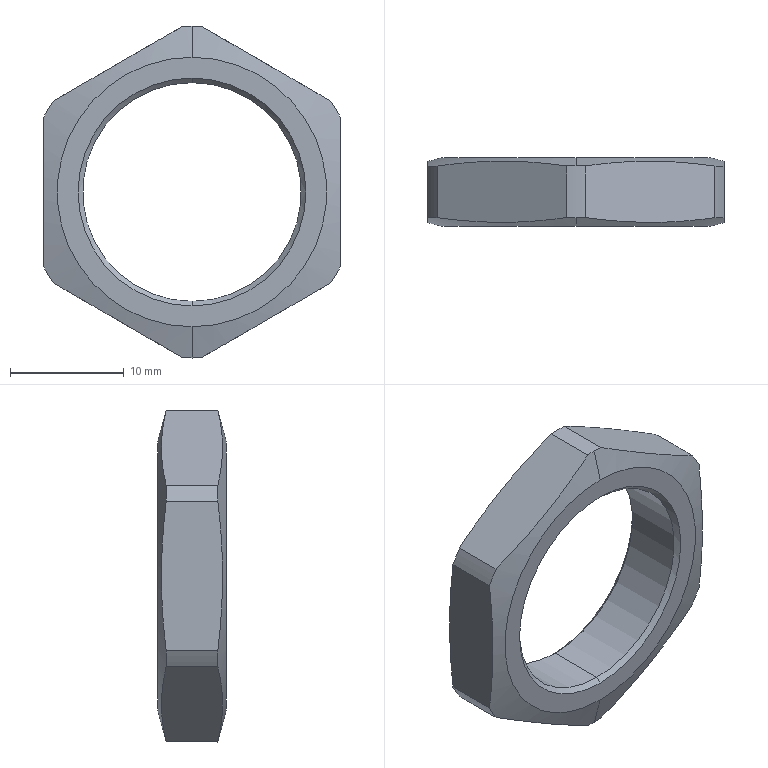Part | SolidWorks | features BaseBody 1 | 1 solid | 25 faces | box 26 x 6 x 29.132 mm | volume 1676 mm3 | cylinder 9 | cone 8 | plane 8 | commonest cylinder face diameters 29.132 x7 19.188 x2
STEP:
#1=CARTESIAN_POINT('',(0.,6.,-11.818));
#2=VERTEX_POINT('',#1);
#3=CARTESIAN_POINT('',(0.,6.,11.818));
#4=VERTEX_POINT('',#3);
#5=CARTESIAN_POINT('',(0.,6.,0.));
#6=DIRECTION('',(0.,-1.,0.));
#7=DIRECTION('',(0.,0.,-1.));
#8=AXIS2_PLACEMENT_3D('',#5,#6,#7);
#9=CIRCLE('',#8,11.818);
#10=EDGE_CURVE('',#2,#4,#9,.T.);
#11=ORIENTED_EDGE('',*,*,#10,.T.);
#12=CARTESIAN_POINT('',(0.,5.264,14.566));
#13=VERTEX_POINT('',#12);
#14=CARTESIAN_POINT('',(0.,3.,23.014));
#15=DIRECTION('',(0.,-0.2588,0.9659));
#16=VECTOR('',#15,1000.);
#17=LINE('',#14,#16);
#18=EDGE_CURVE('',#4,#13,#17,.T.);
#19=ORIENTED_EDGE('',*,*,#18,.T.);
#20=CARTESIAN_POINT('',(0.8103,5.264,14.543));
#21=VERTEX_POINT('',#20);
#22=CARTESIAN_POINT('',(0.,5.264,0.));
#23=DIRECTION('',(0.,-1.,0.));
#24=DIRECTION('',(0.,0.,-1.));
#25=AXIS2_PLACEMENT_3D('',#22,#23,#24);
#26=CIRCLE('',#25,14.566);
#27=EDGE_CURVE('',#21,#13,#26,.T.);
#28=ORIENTED_EDGE('',*,*,#27,.F.);
#29=CARTESIAN_POINT('',(12.19,5.264,7.973));
#30=VERTEX_POINT('',#29);
#31=CARTESIAN_POINT('',(12.19,5.264,7.973));
#32=CARTESIAN_POINT('',(11.241,5.396,8.521));
#33=CARTESIAN_POINT('',(10.293,5.502,9.068));
#34=CARTESIAN_POINT('',(8.397,5.646,10.163));
#35=CARTESIAN_POINT('',(6.5,5.721,11.258));
#36=CARTESIAN_POINT('',(4.603,5.646,12.353));
#37=CARTESIAN_POINT('',(2.707,5.502,13.448));
#38=CARTESIAN_POINT('',(1.759,5.396,13.996));
#39=CARTESIAN_POINT('',(0.8103,5.264,14.543));
#40=B_SPLINE_CURVE_WITH_KNOTS('',3,(#31,#32,#33,#34,#35,#36,#37,#38,#39),.UNSPECIFIED.,.F.,.F.,(4,2,1,2,4),(0.,0.003285,0.00657,0.009855,0.01314),.UNSPECIFIED.);
#41=EDGE_CURVE('',#30,#21,#40,.T.);
#42=ORIENTED_EDGE('',*,*,#41,.F.);
#43=CARTESIAN_POINT('',(13.,5.264,6.57));
#44=VERTEX_POINT('',#43);
#45=CARTESIAN_POINT('',(0.,5.264,0.));
#46=DIRECTION('',(0.,-1.,0.));
#47=DIRECTION('',(0.,0.,-1.));
#48=AXIS2_PLACEMENT_3D('',#45,#46,#47);
#49=CIRCLE('',#48,14.566);
#50=EDGE_CURVE('',#44,#30,#49,.T.);
#51=ORIENTED_EDGE('',*,*,#50,.F.);
#52=CARTESIAN_POINT('',(13.,5.264,-6.57));
#53=VERTEX_POINT('',#52);
#54=CARTESIAN_POINT('',(13.,5.264,-6.57));
#55=CARTESIAN_POINT('',(13.,5.396,-5.475));
#56=CARTESIAN_POINT('',(13.,5.502,-4.38));
#57=CARTESIAN_POINT('',(13.,5.646,-2.19));
#58=CARTESIAN_POINT('',(13.,5.721,0.));
#59=CARTESIAN_POINT('',(13.,5.646,2.19));
#60=CARTESIAN_POINT('',(13.,5.502,4.38));
#61=CARTESIAN_POINT('',(13.,5.396,5.475));
#62=CARTESIAN_POINT('',(13.,5.264,6.57));
#63=B_SPLINE_CURVE_WITH_KNOTS('',3,(#54,#55,#56,#57,#58,#59,#60,#61,#62),.UNSPECIFIED.,.F.,.F.,(4,2,1,2,4),(0.,0.003285,0.00657,0.009855,0.01314),.UNSPECIFIED.);
#64=EDGE_CURVE('',#53,#44,#63,.T.);
#65=ORIENTED_EDGE('',*,*,#64,.F.);
#66=CARTESIAN_POINT('',(12.19,5.264,-7.973));
#67=VERTEX_POINT('',#66);
#68=CARTESIAN_POINT('',(0.,5.264,0.));
#69=DIRECTION('',(0.,-1.,0.));
#70=DIRECTION('',(0.,0.,-1.));
#71=AXIS2_PLACEMENT_3D('',#68,#69,#70);
#72=CIRCLE('',#71,14.566);
#73=EDGE_CURVE('',#67,#53,#72,.T.);
#74=ORIENTED_EDGE('',*,*,#73,.F.);
#75=CARTESIAN_POINT('',(0.8103,5.264,-14.543));
#76=VERTEX_POINT('',#75);
#77=CARTESIAN_POINT('',(0.8103,5.264,-14.543));
#78=CARTESIAN_POINT('',(1.759,5.396,-13.996));
#79=CARTESIAN_POINT('',(2.707,5.502,-13.448));
#80=CARTESIAN_POINT('',(4.603,5.646,-12.353));
#81=CARTESIAN_POINT('',(6.5,5.721,-11.258));
#82=CARTESIAN_POINT('',(8.397,5.646,-10.163));
#83=CARTESIAN_POINT('',(10.293,5.502,-9.068));
#84=CARTESIAN_POINT('',(11.241,5.396,-8.521));
#85=CARTESIAN_POINT('',(12.19,5.264,-7.973));
#86=B_SPLINE_CURVE_WITH_KNOTS('',3,(#77,#78,#79,#80,#81,#82,#83,#84,#85),.UNSPECIFIED.,.F.,.F.,(4,2,1,2,4),(0.,0.003285,0.00657,0.009855,0.01314),.UNSPECIFIED.);
#87=EDGE_CURVE('',#76,#67,#86,.T.);
#88=ORIENTED_EDGE('',*,*,#87,.F.);
#89=CARTESIAN_POINT('',(0.,5.264,-14.566));
#90=VERTEX_POINT('',#89);
#91=CARTESIAN_POINT('',(0.,5.264,0.));
#92=DIRECTION('',(0.,-1.,0.));
#93=DIRECTION('',(0.,0.,-1.));
#94=AXIS2_PLACEMENT_3D('',#91,#92,#93);
#95=CIRCLE('',#94,14.566);
#96=EDGE_CURVE('',#90,#76,#95,.T.);
#97=ORIENTED_EDGE('',*,*,#96,.F.);
#98=CARTESIAN_POINT('',(0.,3.,-23.014));
#99=DIRECTION('',(0.,-0.2588,-0.9659));
#100=VECTOR('',#99,1000.);
#101=LINE('',#98,#100);
#102=EDGE_CURVE('',#2,#90,#101,.T.);
#103=ORIENTED_EDGE('',*,*,#102,.F.);
#104=EDGE_LOOP('',(#11,#19,#28,#42,#51,#65,#74,#88,#97,#103));
#105=FACE_OUTER_BOUND('',#104,.T.);
#106=CARTESIAN_POINT('',(0.,3.,0.));
#107=DIRECTION('',(0.,-1.,0.));
#108=DIRECTION('',(0.,0.,-1.));
#109=AXIS2_PLACEMENT_3D('',#106,#107,#108);
#110=CONICAL_SURFACE('',#109,23.014,1.309);
#111=ADVANCED_FACE('',(#105),#110,.T.);
#112=CARTESIAN_POINT('',(0.,0.406,9.594));
#113=VERTEX_POINT('',#112);
#114=CARTESIAN_POINT('',(0.,0.406,-9.594));
#115=VERTEX_POINT('',#114);
#116=CARTESIAN_POINT('',(0.,0.406,0.));
#117=DIRECTION('',(0.,-1.,0.));
#118=DIRECTION('',(0.,0.,-1.));
#119=AXIS2_PLACEMENT_3D('',#116,#117,#118);
#120=CIRCLE('',#119,9.594);
#121=EDGE_CURVE('',#113,#115,#120,.T.);
#122=ORIENTED_EDGE('',*,*,#121,.F.);
#123=CARTESIAN_POINT('',(0.,0.,10.));
#124=VERTEX_POINT('',#123);
#125=CARTESIAN_POINT('',(0.,0.406,9.594));
#126=DIRECTION('',(0.,-0.7071,0.7071));
#127=VECTOR('',#126,1000.);
#128=LINE('',#125,#127);
#129=EDGE_CURVE('',#113,#124,#128,.T.);
#130=ORIENTED_EDGE('',*,*,#129,.T.);
#131=CARTESIAN_POINT('',(0.,0.,-10.));
#132=VERTEX_POINT('',#131);
#133=CARTESIAN_POINT('',(0.,0.,0.));
#134=DIRECTION('',(0.,-1.,0.));
#135=DIRECTION('',(0.,0.,-1.));
#136=AXIS2_PLACEMENT_3D('',#133,#134,#135);
#137=CIRCLE('',#136,10.);
#138=EDGE_CURVE('',#124,#132,#137,.T.);
#139=ORIENTED_EDGE('',*,*,#138,.T.);
#140=CARTESIAN_POINT('',(0.,0.406,-9.594));
#141=DIRECTION('',(0.,-0.7071,-0.7071));
#142=VECTOR('',#141,1000.);
#143=LINE('',#140,#142);
#144=EDGE_CURVE('',#115,#132,#143,.T.);
#145=ORIENTED_EDGE('',*,*,#144,.F.);
#146=EDGE_LOOP('',(#122,#130,#139,#145));
#147=FACE_OUTER_BOUND('',#146,.T.);
#148=CARTESIAN_POINT('',(0.,0.406,0.));
#149=DIRECTION('',(0.,-1.,0.));
#150=DIRECTION('',(0.,0.,-1.));
#151=AXIS2_PLACEMENT_3D('',#148,#149,#150);
#152=CONICAL_SURFACE('',#151,9.594,0.7854);
#153=ADVANCED_FACE('',(#147),#152,.F.);
#154=CARTESIAN_POINT('',(0.,0.406,0.));
#155=DIRECTION('',(0.,-1.,0.));
#156=DIRECTION('',(0.,0.,-1.));
#157=AXIS2_PLACEMENT_3D('',#154,#155,#156);
#158=CIRCLE('',#157,9.594);
#159=EDGE_CURVE('',#115,#113,#158,.T.);
#160=ORIENTED_EDGE('',*,*,#159,.T.);
#161=CARTESIAN_POINT('',(0.,5.594,9.594));
#162=VERTEX_POINT('',#161);
#163=CARTESIAN_POINT('',(0.,0.,9.594));
#164=DIRECTION('',(0.,1.,0.));
#165=VECTOR('',#164,1000.);
#166=LINE('',#163,#165);
#167=EDGE_CURVE('',#113,#162,#166,.T.);
#168=ORIENTED_EDGE('',*,*,#167,.T.);
#169=CARTESIAN_POINT('',(0.,5.594,-9.594));
#170=VERTEX_POINT('',#169);
#171=CARTESIAN_POINT('',(0.,5.594,0.));
#172=DIRECTION('',(0.,-1.,0.));
#173=DIRECTION('',(0.,0.,-1.));
#174=AXIS2_PLACEMENT_3D('',#171,#172,#173);
#175=CIRCLE('',#174,9.594);
#176=EDGE_CURVE('',#170,#162,#175,.T.);
#177=ORIENTED_EDGE('',*,*,#176,.F.);
#178=CARTESIAN_POINT('',(0.,0.,-9.594));
#179=DIRECTION('',(0.,1.,0.));
#180=VECTOR('',#179,1000.);
#181=LINE('',#178,#180);
#182=EDGE_CURVE('',#115,#170,#181,.T.);
#183=ORIENTED_EDGE('',*,*,#182,.F.);
#184=EDGE_LOOP('',(#160,#168,#177,#183));
#185=FACE_OUTER_BOUND('',#184,.T.);
#186=CARTESIAN_POINT('',(0.,0.,0.));
#187=DIRECTION('',(0.,1.,0.));
#188=DIRECTION('',(0.,0.,-1.));
#189=AXIS2_PLACEMENT_3D('',#186,#187,#188);
#190=CYLINDRICAL_SURFACE('',#189,9.594);
#191=ADVANCED_FACE('',(#185),#190,.F.);
#192=CARTESIAN_POINT('',(0.,5.594,0.));
#193=DIRECTION('',(0.,-1.,0.));
#194=DIRECTION('',(0.,0.,-1.));
#195=AXIS2_PLACEMENT_3D('',#192,#193,#194);
#196=CIRCLE('',#195,9.594);
#197=EDGE_CURVE('',#162,#170,#196,.T.);
#198=ORIENTED_EDGE('',*,*,#197,.T.);
#199=CARTESIAN_POINT('',(0.,6.,-10.));
#200=VERTEX_POINT('',#199);
#201=CARTESIAN_POINT('',(0.,6.,-10.));
#202=DIRECTION('',(0.,0.7071,-0.7071));
#203=VECTOR('',#202,1000.);
#204=LINE('',#201,#203);
#205=EDGE_CURVE('',#170,#200,#204,.T.);
#206=ORIENTED_EDGE('',*,*,#205,.T.);
#207=CARTESIAN_POINT('',(0.,6.,10.));
#208=VERTEX_POINT('',#207);
#209=CARTESIAN_POINT('',(0.,6.,0.));
#210=DIRECTION('',(0.,-1.,0.));
#211=DIRECTION('',(0.,0.,-1.));
#212=AXIS2_PLACEMENT_3D('',#209,#210,#211);
#213=CIRCLE('',#212,10.);
#214=EDGE_CURVE('',#208,#200,#213,.T.);
#215=ORIENTED_EDGE('',*,*,#214,.F.);
#216=CARTESIAN_POINT('',(0.,6.,10.));
#217=DIRECTION('',(0.,0.7071,0.7071));
#218=VECTOR('',#217,1000.);
#219=LINE('',#216,#218);
#220=EDGE_CURVE('',#162,#208,#219,.T.);
#221=ORIENTED_EDGE('',*,*,#220,.F.);
#222=EDGE_LOOP('',(#198,#206,#215,#221));
#223=FACE_OUTER_BOUND('',#222,.T.);
#224=CARTESIAN_POINT('',(0.,6.,0.));
#225=DIRECTION('',(0.,1.,0.));
#226=DIRECTION('',(0.,0.,1.));
#227=AXIS2_PLACEMENT_3D('',#224,#225,#226);
#228=CONICAL_SURFACE('',#227,10.,0.7854);
#229=ADVANCED_FACE('',(#223),#228,.F.);
#230=CARTESIAN_POINT('',(0.8103,0.7362,-14.543));
#231=VERTEX_POINT('',#230);
#232=CARTESIAN_POINT('',(0.,0.7362,-14.566));
#233=VERTEX_POINT('',#232);
#234=CARTESIAN_POINT('',(0.,0.7362,0.));
#235=DIRECTION('',(0.,1.,0.));
#236=DIRECTION('',(0.,0.,1.));
#237=AXIS2_PLACEMENT_3D('',#234,#235,#236);
#238=CIRCLE('',#237,14.566);
#239=EDGE_CURVE('',#231,#233,#238,.T.);
#240=ORIENTED_EDGE('',*,*,#239,.T.);
#241=CARTESIAN_POINT('',(0.,6.,-14.566));
#242=DIRECTION('',(0.,1.,0.));
#243=VECTOR('',#242,1000.);
#244=LINE('',#241,#243);
#245=EDGE_CURVE('',#233,#90,#244,.T.);
#246=ORIENTED_EDGE('',*,*,#245,.T.);
#247=ORIENTED_EDGE('',*,*,#96,.T.);
#248=CARTESIAN_POINT('',(0.8103,6.,-14.543));
#249=DIRECTION('',(0.,1.,0.));
#250=VECTOR('',#249,1000.);
#251=LINE('',#248,#250);
#252=EDGE_CURVE('',#231,#76,#251,.T.);
#253=ORIENTED_EDGE('',*,*,#252,.F.);
#254=EDGE_LOOP('',(#240,#246,#247,#253));
#255=FACE_OUTER_BOUND('',#254,.T.);
#256=CARTESIAN_POINT('',(0.,6.,0.));
#257=DIRECTION('',(0.,1.,0.));
#258=DIRECTION('',(0.,0.,-1.));
#259=AXIS2_PLACEMENT_3D('',#256,#257,#258);
#260=CYLINDRICAL_SURFACE('',#259,14.566);
#261=ADVANCED_FACE('',(#255),#260,.T.);
#262=CARTESIAN_POINT('',(0.,0.,-11.818));
#263=VERTEX_POINT('',#262);
#264=CARTESIAN_POINT('',(0.,0.,11.818));
#265=VERTEX_POINT('',#264);
#266=CARTESIAN_POINT('',(0.,0.,0.));
#267=DIRECTION('',(0.,-1.,0.));
#268=DIRECTION('',(0.,0.,-1.));
#269=AXIS2_PLACEMENT_3D('',#266,#267,#268);
#270=CIRCLE('',#269,11.818);
#271=EDGE_CURVE('',#263,#265,#270,.T.);
#272=ORIENTED_EDGE('',*,*,#271,.F.);
#273=CARTESIAN_POINT('',(0.,0.,-11.818));
#274=DIRECTION('',(0.,0.2588,-0.9659));
#275=VECTOR('',#274,1000.);
#276=LINE('',#273,#275);
#277=EDGE_CURVE('',#263,#233,#276,.T.);
#278=ORIENTED_EDGE('',*,*,#277,.T.);
#279=ORIENTED_EDGE('',*,*,#239,.F.);
#280=CARTESIAN_POINT('',(12.19,0.7362,-7.973));
#281=VERTEX_POINT('',#280);
#282=CARTESIAN_POINT('',(12.19,0.7362,-7.973));
#283=CARTESIAN_POINT('',(11.241,0.6039,-8.521));
#284=CARTESIAN_POINT('',(10.293,0.498,-9.068));
#285=CARTESIAN_POINT('',(8.397,0.3543,-10.163));
#286=CARTESIAN_POINT('',(6.5,0.2791,-11.258));
#287=CARTESIAN_POINT('',(4.603,0.3543,-12.353));
#288=CARTESIAN_POINT('',(2.707,0.498,-13.448));
#289=CARTESIAN_POINT('',(1.759,0.6039,-13.996));
#290=CARTESIAN_POINT('',(0.8103,0.7362,-14.543));
#291=B_SPLINE_CURVE_WITH_KNOTS('',3,(#282,#283,#284,#285,#286,#287,#288,#289,#290),.UNSPECIFIED.,.F.,.F.,(4,2,1,2,4),(0.,0.003285,0.00657,0.009855,0.01314),.UNSPECIFIED.);
#292=EDGE_CURVE('',#281,#231,#291,.T.);
#293=ORIENTED_EDGE('',*,*,#292,.F.);
#294=CARTESIAN_POINT('',(13.,0.7362,-6.57));
#295=VERTEX_POINT('',#294);
#296=CARTESIAN_POINT('',(0.,0.7362,0.));
#297=DIRECTION('',(0.,1.,0.));
#298=DIRECTION('',(0.,0.,1.));
#299=AXIS2_PLACEMENT_3D('',#296,#297,#298);
#300=CIRCLE('',#299,14.566);
#301=EDGE_CURVE('',#295,#281,#300,.T.);
#302=ORIENTED_EDGE('',*,*,#301,.F.);
#303=CARTESIAN_POINT('',(13.,0.7362,6.57));
#304=VERTEX_POINT('',#303);
#305=CARTESIAN_POINT('',(13.,0.7362,6.57));
#306=CARTESIAN_POINT('',(13.,0.6039,5.475));
#307=CARTESIAN_POINT('',(13.,0.498,4.38));
#308=CARTESIAN_POINT('',(13.,0.3543,2.19));
#309=CARTESIAN_POINT('',(13.,0.2791,0.));
#310=CARTESIAN_POINT('',(13.,0.3543,-2.19));
#311=CARTESIAN_POINT('',(13.,0.498,-4.38));
#312=CARTESIAN_POINT('',(13.,0.6039,-5.475));
#313=CARTESIAN_POINT('',(13.,0.7362,-6.57));
#314=B_SPLINE_CURVE_WITH_KNOTS('',3,(#305,#306,#307,#308,#309,#310,#311,#312,#313),.UNSPECIFIED.,.F.,.F.,(4,2,1,2,4),(0.,0.003285,0.00657,0.009855,0.01314),.UNSPECIFIED.);
#315=EDGE_CURVE('',#304,#295,#314,.T.);
#316=ORIENTED_EDGE('',*,*,#315,.F.);
#317=CARTESIAN_POINT('',(12.19,0.7362,7.973));
#318=VERTEX_POINT('',#317);
#319=CARTESIAN_POINT('',(0.,0.7362,0.));
#320=DIRECTION('',(0.,1.,0.));
#321=DIRECTION('',(0.,0.,1.));
#322=AXIS2_PLACEMENT_3D('',#319,#320,#321);
#323=CIRCLE('',#322,14.566);
#324=EDGE_CURVE('',#318,#304,#323,.T.);
#325=ORIENTED_EDGE('',*,*,#324,.F.);
#326=CARTESIAN_POINT('',(0.8103,0.7362,14.543));
#327=VERTEX_POINT('',#326);
#328=CARTESIAN_POINT('',(0.8103,0.7362,14.543));
#329=CARTESIAN_POINT('',(1.759,0.6039,13.996));
#330=CARTESIAN_POINT('',(2.707,0.498,13.448));
#331=CARTESIAN_POINT('',(4.603,0.3543,12.353));
#332=CARTESIAN_POINT('',(6.5,0.2791,11.258));
#333=CARTESIAN_POINT('',(8.397,0.3543,10.163));
#334=CARTESIAN_POINT('',(10.293,0.498,9.068));
#335=CARTESIAN_POINT('',(11.241,0.6039,8.521));
#336=CARTESIAN_POINT('',(12.19,0.7362,7.973));
#337=B_SPLINE_CURVE_WITH_KNOTS('',3,(#328,#329,#330,#331,#332,#333,#334,#335,#336),.UNSPECIFIED.,.F.,.F.,(4,2,1,2,4),(0.,0.003285,0.00657,0.009855,0.01314),.UNSPECIFIED.);
#338=EDGE_CURVE('',#327,#318,#337,.T.);
#339=ORIENTED_EDGE('',*,*,#338,.F.);
#340=CARTESIAN_POINT('',(0.,0.7362,14.566));
#341=VERTEX_POINT('',#340);
#342=CARTESIAN_POINT('',(0.,0.7362,0.));
#343=DIRECTION('',(0.,1.,0.));
#344=DIRECTION('',(0.,0.,1.));
#345=AXIS2_PLACEMENT_3D('',#342,#343,#344);
#346=CIRCLE('',#345,14.566);
#347=EDGE_CURVE('',#341,#327,#346,.T.);
#348=ORIENTED_EDGE('',*,*,#347,.F.);
#349=CARTESIAN_POINT('',(0.,0.,11.818));
#350=DIRECTION('',(0.,0.2588,0.9659));
#351=VECTOR('',#350,1000.);
#352=LINE('',#349,#351);
#353=EDGE_CURVE('',#265,#341,#352,.T.);
#354=ORIENTED_EDGE('',*,*,#353,.F.);
#355=EDGE_LOOP('',(#272,#278,#279,#293,#302,#316,#325,#339,#348,#354));
#356=FACE_OUTER_BOUND('',#355,.T.);
#357=CARTESIAN_POINT('',(0.,0.,0.));
#358=DIRECTION('',(0.,1.,0.));
#359=DIRECTION('',(0.,0.,1.));
#360=AXIS2_PLACEMENT_3D('',#357,#358,#359);
#361=CONICAL_SURFACE('',#360,11.818,1.309);
#362=ADVANCED_FACE('',(#356),#361,.T.);
#363=ORIENTED_EDGE('',*,*,#277,.F.);
#364=CARTESIAN_POINT('',(0.,0.,0.));
#365=DIRECTION('',(0.,-1.,0.));
#366=DIRECTION('',(0.,0.,-1.));
#367=AXIS2_PLACEMENT_3D('',#364,#365,#366);
#368=CIRCLE('',#367,11.818);
#369=EDGE_CURVE('',#265,#263,#368,.T.);
#370=ORIENTED_EDGE('',*,*,#369,.F.);
#371=ORIENTED_EDGE('',*,*,#353,.T.);
#372=CARTESIAN_POINT('',(-0.8103,0.7362,14.543));
#373=VERTEX_POINT('',#372);
#374=CARTESIAN_POINT('',(0.,0.7362,0.));
#375=DIRECTION('',(0.,1.,0.));
#376=DIRECTION('',(0.,0.,1.));
#377=AXIS2_PLACEMENT_3D('',#374,#375,#376);
#378=CIRCLE('',#377,14.566);
#379=EDGE_CURVE('',#373,#341,#378,.T.);
#380=ORIENTED_EDGE('',*,*,#379,.F.);
#381=CARTESIAN_POINT('',(-12.19,0.7362,7.973));
#382=VERTEX_POINT('',#381);
#383=CARTESIAN_POINT('',(-12.19,0.7362,7.973));
#384=CARTESIAN_POINT('',(-11.241,0.6039,8.521));
#385=CARTESIAN_POINT('',(-10.293,0.498,9.068));
#386=CARTESIAN_POINT('',(-8.397,0.3543,10.163));
#387=CARTESIAN_POINT('',(-6.5,0.2791,11.258));
#388=CARTESIAN_POINT('',(-4.603,0.3543,12.353));
#389=CARTESIAN_POINT('',(-2.707,0.498,13.448));
#390=CARTESIAN_POINT('',(-1.759,0.6039,13.996));
#391=CARTESIAN_POINT('',(-0.8103,0.7362,14.543));
#392=B_SPLINE_CURVE_WITH_KNOTS('',3,(#383,#384,#385,#386,#387,#388,#389,#390,#391),.UNSPECIFIED.,.F.,.F.,(4,2,1,2,4),(0.,0.003285,0.00657,0.009855,0.01314),.UNSPECIFIED.);
#393=EDGE_CURVE('',#382,#373,#392,.T.);
#394=ORIENTED_EDGE('',*,*,#393,.F.);
#395=CARTESIAN_POINT('',(-13.,0.7362,6.57));
#396=VERTEX_POINT('',#395);
#397=CARTESIAN_POINT('',(0.,0.7362,0.));
#398=DIRECTION('',(0.,1.,0.));
#399=DIRECTION('',(0.,0.,1.));
#400=AXIS2_PLACEMENT_3D('',#397,#398,#399);
#401=CIRCLE('',#400,14.566);
#402=EDGE_CURVE('',#396,#382,#401,.T.);
#403=ORIENTED_EDGE('',*,*,#402,.F.);
#404=CARTESIAN_POINT('',(-13.,0.7362,-6.57));
#405=VERTEX_POINT('',#404);
#406=CARTESIAN_POINT('',(-13.,0.7362,-6.57));
#407=CARTESIAN_POINT('',(-13.,0.6039,-5.475));
#408=CARTESIAN_POINT('',(-13.,0.498,-4.38));
#409=CARTESIAN_POINT('',(-13.,0.3543,-2.19));
#410=CARTESIAN_POINT('',(-13.,0.2791,0.));
#411=CARTESIAN_POINT('',(-13.,0.3543,2.19));
#412=CARTESIAN_POINT('',(-13.,0.498,4.38));
#413=CARTESIAN_POINT('',(-13.,0.6039,5.475));
#414=CARTESIAN_POINT('',(-13.,0.7362,6.57));
#415=B_SPLINE_CURVE_WITH_KNOTS('',3,(#406,#407,#408,#409,#410,#411,#412,#413,#414),.UNSPECIFIED.,.F.,.F.,(4,2,1,2,4),(0.,0.003285,0.00657,0.009855,0.01314),.UNSPECIFIED.);
#416=EDGE_CURVE('',#405,#396,#415,.T.);
#417=ORIENTED_EDGE('',*,*,#416,.F.);
#418=CARTESIAN_POINT('',(-12.19,0.7362,-7.973));
#419=VERTEX_POINT('',#418);
#420=CARTESIAN_POINT('',(0.,0.7362,0.));
#421=DIRECTION('',(0.,1.,0.));
#422=DIRECTION('',(0.,0.,1.));
#423=AXIS2_PLACEMENT_3D('',#420,#421,#422);
#424=CIRCLE('',#423,14.566);
#425=EDGE_CURVE('',#419,#405,#424,.T.);
#426=ORIENTED_EDGE('',*,*,#425,.F.);
#427=CARTESIAN_POINT('',(-0.8103,0.7362,-14.543));
#428=VERTEX_POINT('',#427);
#429=CARTESIAN_POINT('',(-0.8103,0.7362,-14.543));
#430=CARTESIAN_POINT('',(-1.759,0.6039,-13.996));
#431=CARTESIAN_POINT('',(-2.707,0.498,-13.448));
#432=CARTESIAN_POINT('',(-4.603,0.3543,-12.353));
#433=CARTESIAN_POINT('',(-6.5,0.2791,-11.258));
#434=CARTESIAN_POINT('',(-8.397,0.3543,-10.163));
#435=CARTESIAN_POINT('',(-10.293,0.498,-9.068));
#436=CARTESIAN_POINT('',(-11.241,0.6039,-8.521));
#437=CARTESIAN_POINT('',(-12.19,0.7362,-7.973));
#438=B_SPLINE_CURVE_WITH_KNOTS('',3,(#429,#430,#431,#432,#433,#434,#435,#436,#437),.UNSPECIFIED.,.F.,.F.,(4,2,1,2,4),(0.,0.003285,0.00657,0.009855,0.01314),.UNSPECIFIED.);
#439=EDGE_CURVE('',#428,#419,#438,.T.);
#440=ORIENTED_EDGE('',*,*,#439,.F.);
#441=CARTESIAN_POINT('',(0.,0.7362,0.));
#442=DIRECTION('',(0.,1.,0.));
#443=DIRECTION('',(0.,0.,1.));
#444=AXIS2_PLACEMENT_3D('',#441,#442,#443);
#445=CIRCLE('',#444,14.566);
#446=EDGE_CURVE('',#233,#428,#445,.T.);
#447=ORIENTED_EDGE('',*,*,#446,.F.);
#448=EDGE_LOOP('',(#363,#370,#371,#380,#394,#403,#417,#426,#440,#447));
#449=FACE_OUTER_BOUND('',#448,.T.);
#450=CARTESIAN_POINT('',(0.,0.,0.));
#451=DIRECTION('',(0.,1.,0.));
#452=DIRECTION('',(0.,0.,1.));
#453=AXIS2_PLACEMENT_3D('',#450,#451,#452);
#454=CONICAL_SURFACE('',#453,11.818,1.309);
#455=ADVANCED_FACE('',(#449),#454,.T.);
#456=ORIENTED_EDGE('',*,*,#416,.T.);
#457=CARTESIAN_POINT('',(-13.,5.264,6.57));
#458=VERTEX_POINT('',#457);
#459=CARTESIAN_POINT('',(-13.,6.,6.57));
#460=DIRECTION('',(0.,1.,0.));
#461=VECTOR('',#460,1000.);
#462=LINE('',#459,#461);
#463=EDGE_CURVE('',#396,#458,#462,.T.);
#464=ORIENTED_EDGE('',*,*,#463,.T.);
#465=CARTESIAN_POINT('',(-13.,5.264,-6.57));
#466=VERTEX_POINT('',#465);
#467=CARTESIAN_POINT('',(-13.,5.264,6.57));
#468=CARTESIAN_POINT('',(-13.,5.396,5.475));
#469=CARTESIAN_POINT('',(-13.,5.502,4.38));
#470=CARTESIAN_POINT('',(-13.,5.646,2.19));
#471=CARTESIAN_POINT('',(-13.,5.721,0.));
#472=CARTESIAN_POINT('',(-13.,5.646,-2.19));
#473=CARTESIAN_POINT('',(-13.,5.502,-4.38));
#474=CARTESIAN_POINT('',(-13.,5.396,-5.475));
#475=CARTESIAN_POINT('',(-13.,5.264,-6.57));
#476=B_SPLINE_CURVE_WITH_KNOTS('',3,(#467,#468,#469,#470,#471,#472,#473,#474,#475),.UNSPECIFIED.,.F.,.F.,(4,2,1,2,4),(0.,0.003285,0.00657,0.009855,0.01314),.UNSPECIFIED.);
#477=EDGE_CURVE('',#458,#466,#476,.T.);
#478=ORIENTED_EDGE('',*,*,#477,.T.);
#479=CARTESIAN_POINT('',(-13.,6.,-6.57));
#480=DIRECTION('',(0.,-1.,0.));
#481=VECTOR('',#480,1000.);
#482=LINE('',#479,#481);
#483=EDGE_CURVE('',#466,#405,#482,.T.);
#484=ORIENTED_EDGE('',*,*,#483,.T.);
#485=EDGE_LOOP('',(#456,#464,#478,#484));
#486=FACE_OUTER_BOUND('',#485,.T.);
#487=CARTESIAN_POINT('',(-13.,6.,-7.506));
#488=DIRECTION('',(1.,0.,0.));
#489=DIRECTION('',(0.,1.,0.));
#490=AXIS2_PLACEMENT_3D('',#487,#488,#489);
#491=PLANE('',#490);
#492=ADVANCED_FACE('',(#486),#491,.F.);
#493=ORIENTED_EDGE('',*,*,#425,.T.);
#494=ORIENTED_EDGE('',*,*,#483,.F.);
#495=CARTESIAN_POINT('',(-12.19,5.264,-7.973));
#496=VERTEX_POINT('',#495);
#497=CARTESIAN_POINT('',(0.,5.264,0.));
#498=DIRECTION('',(0.,-1.,0.));
#499=DIRECTION('',(0.,0.,-1.));
#500=AXIS2_PLACEMENT_3D('',#497,#498,#499);
#501=CIRCLE('',#500,14.566);
#502=EDGE_CURVE('',#466,#496,#501,.T.);
#503=ORIENTED_EDGE('',*,*,#502,.T.);
#504=CARTESIAN_POINT('',(-12.19,6.,-7.973));
#505=DIRECTION('',(0.,1.,0.));
#506=VECTOR('',#505,1000.);
#507=LINE('',#504,#506);
#508=EDGE_CURVE('',#419,#496,#507,.T.);
#509=ORIENTED_EDGE('',*,*,#508,.F.);
#510=EDGE_LOOP('',(#493,#494,#503,#509));
#511=FACE_OUTER_BOUND('',#510,.T.);
#512=CARTESIAN_POINT('',(0.,6.,0.));
#513=DIRECTION('',(0.,1.,0.));
#514=DIRECTION('',(0.,0.,-1.));
#515=AXIS2_PLACEMENT_3D('',#512,#513,#514);
#516=CYLINDRICAL_SURFACE('',#515,14.566);
#517=ADVANCED_FACE('',(#511),#516,.T.);
#518=CARTESIAN_POINT('',(-12.19,5.264,7.973));
#519=VERTEX_POINT('',#518);
#520=CARTESIAN_POINT('',(0.,5.264,0.));
#521=DIRECTION('',(0.,-1.,0.));
#522=DIRECTION('',(0.,0.,-1.));
#523=AXIS2_PLACEMENT_3D('',#520,#521,#522);
#524=CIRCLE('',#523,14.566);
#525=EDGE_CURVE('',#519,#458,#524,.T.);
#526=ORIENTED_EDGE('',*,*,#525,.T.);
#527=ORIENTED_EDGE('',*,*,#463,.F.);
#528=ORIENTED_EDGE('',*,*,#402,.T.);
#529=CARTESIAN_POINT('',(-12.19,6.,7.973));
#530=DIRECTION('',(0.,-1.,0.));
#531=VECTOR('',#530,1000.);
#532=LINE('',#529,#531);
#533=EDGE_CURVE('',#519,#382,#532,.T.);
#534=ORIENTED_EDGE('',*,*,#533,.F.);
#535=EDGE_LOOP('',(#526,#527,#528,#534));
#536=FACE_OUTER_BOUND('',#535,.T.);
#537=CARTESIAN_POINT('',(0.,6.,0.));
#538=DIRECTION('',(0.,1.,0.));
#539=DIRECTION('',(0.,0.,-1.));
#540=AXIS2_PLACEMENT_3D('',#537,#538,#539);
#541=CYLINDRICAL_SURFACE('',#540,14.566);
#542=ADVANCED_FACE('',(#536),#541,.T.);
#543=ORIENTED_EDGE('',*,*,#27,.T.);
#544=CARTESIAN_POINT('',(-0.8103,5.264,14.543));
#545=VERTEX_POINT('',#544);
#546=CARTESIAN_POINT('',(0.,5.264,0.));
#547=DIRECTION('',(0.,-1.,0.));
#548=DIRECTION('',(0.,0.,-1.));
#549=AXIS2_PLACEMENT_3D('',#546,#547,#548);
#550=CIRCLE('',#549,14.566);
#551=EDGE_CURVE('',#13,#545,#550,.T.);
#552=ORIENTED_EDGE('',*,*,#551,.T.);
#553=CARTESIAN_POINT('',(-0.8103,6.,14.543));
#554=DIRECTION('',(0.,1.,0.));
#555=VECTOR('',#554,1000.);
#556=LINE('',#553,#555);
#557=EDGE_CURVE('',#373,#545,#556,.T.);
#558=ORIENTED_EDGE('',*,*,#557,.F.);
#559=ORIENTED_EDGE('',*,*,#379,.T.);
#560=ORIENTED_EDGE('',*,*,#347,.T.);
#561=CARTESIAN_POINT('',(0.8103,6.,14.543));
#562=DIRECTION('',(0.,-1.,0.));
#563=VECTOR('',#562,1000.);
#564=LINE('',#561,#563);
#565=EDGE_CURVE('',#21,#327,#564,.T.);
#566=ORIENTED_EDGE('',*,*,#565,.F.);
#567=EDGE_LOOP('',(#543,#552,#558,#559,#560,#566));
#568=FACE_OUTER_BOUND('',#567,.T.);
#569=CARTESIAN_POINT('',(0.,6.,0.));
#570=DIRECTION('',(0.,1.,0.));
#571=DIRECTION('',(0.,0.,-1.));
#572=AXIS2_PLACEMENT_3D('',#569,#570,#571);
#573=CYLINDRICAL_SURFACE('',#572,14.566);
#574=ADVANCED_FACE('',(#568),#573,.T.);
#575=ORIENTED_EDGE('',*,*,#50,.T.);
#576=CARTESIAN_POINT('',(12.19,6.,7.973));
#577=DIRECTION('',(0.,1.,0.));
#578=VECTOR('',#577,1000.);
#579=LINE('',#576,#578);
#580=EDGE_CURVE('',#318,#30,#579,.T.);
#581=ORIENTED_EDGE('',*,*,#580,.F.);
#582=ORIENTED_EDGE('',*,*,#324,.T.);
#583=CARTESIAN_POINT('',(13.,6.,6.57));
#584=DIRECTION('',(0.,-1.,0.));
#585=VECTOR('',#584,1000.);
#586=LINE('',#583,#585);
#587=EDGE_CURVE('',#44,#304,#586,.T.);
#588=ORIENTED_EDGE('',*,*,#587,.F.);
#589=EDGE_LOOP('',(#575,#581,#582,#588));
#590=FACE_OUTER_BOUND('',#589,.T.);
#591=CARTESIAN_POINT('',(0.,6.,0.));
#592=DIRECTION('',(0.,1.,0.));
#593=DIRECTION('',(0.,0.,-1.));
#594=AXIS2_PLACEMENT_3D('',#591,#592,#593);
#595=CYLINDRICAL_SURFACE('',#594,14.566);
#596=ADVANCED_FACE('',(#590),#595,.T.);
#597=ORIENTED_EDGE('',*,*,#245,.F.);
#598=ORIENTED_EDGE('',*,*,#446,.T.);
#599=CARTESIAN_POINT('',(-0.8103,5.264,-14.543));
#600=VERTEX_POINT('',#599);
#601=CARTESIAN_POINT('',(-0.8103,6.,-14.543));
#602=DIRECTION('',(0.,-1.,0.));
#603=VECTOR('',#602,1000.);
#604=LINE('',#601,#603);
#605=EDGE_CURVE('',#600,#428,#604,.T.);
#606=ORIENTED_EDGE('',*,*,#605,.F.);
#607=CARTESIAN_POINT('',(0.,5.264,0.));
#608=DIRECTION('',(0.,-1.,0.));
#609=DIRECTION('',(0.,0.,-1.));
#610=AXIS2_PLACEMENT_3D('',#607,#608,#609);
#611=CIRCLE('',#610,14.566);
#612=EDGE_CURVE('',#600,#90,#611,.T.);
#613=ORIENTED_EDGE('',*,*,#612,.T.);
#614=EDGE_LOOP('',(#597,#598,#606,#613));
#615=FACE_OUTER_BOUND('',#614,.T.);
#616=CARTESIAN_POINT('',(0.,6.,0.));
#617=DIRECTION('',(0.,1.,0.));
#618=DIRECTION('',(0.,0.,-1.));
#619=AXIS2_PLACEMENT_3D('',#616,#617,#618);
#620=CYLINDRICAL_SURFACE('',#619,14.566);
#621=ADVANCED_FACE('',(#615),#620,.T.);
#622=ORIENTED_EDGE('',*,*,#73,.T.);
#623=CARTESIAN_POINT('',(13.,6.,-6.57));
#624=DIRECTION('',(0.,1.,0.));
#625=VECTOR('',#624,1000.);
#626=LINE('',#623,#625);
#627=EDGE_CURVE('',#295,#53,#626,.T.);
#628=ORIENTED_EDGE('',*,*,#627,.F.);
#629=ORIENTED_EDGE('',*,*,#301,.T.);
#630=CARTESIAN_POINT('',(12.19,6.,-7.973));
#631=DIRECTION('',(0.,-1.,0.));
#632=VECTOR('',#631,1000.);
#633=LINE('',#630,#632);
#634=EDGE_CURVE('',#67,#281,#633,.T.);
#635=ORIENTED_EDGE('',*,*,#634,.F.);
#636=EDGE_LOOP('',(#622,#628,#629,#635));
#637=FACE_OUTER_BOUND('',#636,.T.);
#638=CARTESIAN_POINT('',(0.,6.,0.));
#639=DIRECTION('',(0.,1.,0.));
#640=DIRECTION('',(0.,0.,-1.));
#641=AXIS2_PLACEMENT_3D('',#638,#639,#640);
#642=CYLINDRICAL_SURFACE('',#641,14.566);
#643=ADVANCED_FACE('',(#637),#642,.T.);
#644=ORIENTED_EDGE('',*,*,#315,.T.);
#645=ORIENTED_EDGE('',*,*,#627,.T.);
#646=ORIENTED_EDGE('',*,*,#64,.T.);
#647=ORIENTED_EDGE('',*,*,#587,.T.);
#648=EDGE_LOOP('',(#644,#645,#646,#647));
#649=FACE_OUTER_BOUND('',#648,.T.);
#650=CARTESIAN_POINT('',(13.,6.,7.506));
#651=DIRECTION('',(-1.,0.,0.));
#652=DIRECTION('',(0.,0.,1.));
#653=AXIS2_PLACEMENT_3D('',#650,#651,#652);
#654=PLANE('',#653);
#655=ADVANCED_FACE('',(#649),#654,.F.);
#656=ORIENTED_EDGE('',*,*,#338,.T.);
#657=ORIENTED_EDGE('',*,*,#580,.T.);
#658=ORIENTED_EDGE('',*,*,#41,.T.);
#659=ORIENTED_EDGE('',*,*,#565,.T.);
#660=EDGE_LOOP('',(#656,#657,#658,#659));
#661=FACE_OUTER_BOUND('',#660,.T.);
#662=CARTESIAN_POINT('',(0.,6.,15.011));
#663=DIRECTION('',(-0.5,0.,-0.866));
#664=DIRECTION('',(-0.866,0.,0.5));
#665=AXIS2_PLACEMENT_3D('',#662,#663,#664);
#666=PLANE('',#665);
#667=ADVANCED_FACE('',(#661),#666,.F.);
#668=ORIENTED_EDGE('',*,*,#393,.T.);
#669=ORIENTED_EDGE('',*,*,#557,.T.);
#670=CARTESIAN_POINT('',(-0.8103,5.264,14.543));
#671=CARTESIAN_POINT('',(-1.759,5.396,13.996));
#672=CARTESIAN_POINT('',(-2.707,5.502,13.448));
#673=CARTESIAN_POINT('',(-4.603,5.646,12.353));
#674=CARTESIAN_POINT('',(-6.5,5.721,11.258));
#675=CARTESIAN_POINT('',(-8.397,5.646,10.163));
#676=CARTESIAN_POINT('',(-10.293,5.502,9.068));
#677=CARTESIAN_POINT('',(-11.241,5.396,8.521));
#678=CARTESIAN_POINT('',(-12.19,5.264,7.973));
#679=B_SPLINE_CURVE_WITH_KNOTS('',3,(#670,#671,#672,#673,#674,#675,#676,#677,#678),.UNSPECIFIED.,.F.,.F.,(4,2,1,2,4),(0.,0.003285,0.00657,0.009855,0.01314),.UNSPECIFIED.);
#680=EDGE_CURVE('',#545,#519,#679,.T.);
#681=ORIENTED_EDGE('',*,*,#680,.T.);
#682=ORIENTED_EDGE('',*,*,#533,.T.);
#683=EDGE_LOOP('',(#668,#669,#681,#682));
#684=FACE_OUTER_BOUND('',#683,.T.);
#685=CARTESIAN_POINT('',(-13.,6.,7.506));
#686=DIRECTION('',(0.5,0.,-0.866));
#687=DIRECTION('',(0.,-1.,0.));
#688=AXIS2_PLACEMENT_3D('',#685,#686,#687);
#689=PLANE('',#688);
#690=ADVANCED_FACE('',(#684),#689,.F.);
#691=ORIENTED_EDGE('',*,*,#439,.T.);
#692=ORIENTED_EDGE('',*,*,#508,.T.);
#693=CARTESIAN_POINT('',(-12.19,5.264,-7.973));
#694=CARTESIAN_POINT('',(-11.241,5.396,-8.521));
#695=CARTESIAN_POINT('',(-10.293,5.502,-9.068));
#696=CARTESIAN_POINT('',(-8.397,5.646,-10.163));
#697=CARTESIAN_POINT('',(-6.5,5.721,-11.258));
#698=CARTESIAN_POINT('',(-4.603,5.646,-12.353));
#699=CARTESIAN_POINT('',(-2.707,5.502,-13.448));
#700=CARTESIAN_POINT('',(-1.759,5.396,-13.996));
#701=CARTESIAN_POINT('',(-0.8103,5.264,-14.543));
#702=B_SPLINE_CURVE_WITH_KNOTS('',3,(#693,#694,#695,#696,#697,#698,#699,#700,#701),.UNSPECIFIED.,.F.,.F.,(4,2,1,2,4),(0.,0.003285,0.00657,0.009855,0.01314),.UNSPECIFIED.);
#703=EDGE_CURVE('',#496,#600,#702,.T.);
#704=ORIENTED_EDGE('',*,*,#703,.T.);
#705=ORIENTED_EDGE('',*,*,#605,.T.);
#706=EDGE_LOOP('',(#691,#692,#704,#705));
#707=FACE_OUTER_BOUND('',#706,.T.);
#708=CARTESIAN_POINT('',(0.,6.,-15.011));
#709=DIRECTION('',(0.5,0.,0.866));
#710=DIRECTION('',(0.,-1.,0.));
#711=AXIS2_PLACEMENT_3D('',#708,#709,#710);
#712=PLANE('',#711);
#713=ADVANCED_FACE('',(#707),#712,.F.);
#714=ORIENTED_EDGE('',*,*,#214,.T.);
#715=CARTESIAN_POINT('',(0.,6.,0.));
#716=DIRECTION('',(0.,-1.,0.));
#717=DIRECTION('',(0.,0.,-1.));
#718=AXIS2_PLACEMENT_3D('',#715,#716,#717);
#719=CIRCLE('',#718,10.);
#720=EDGE_CURVE('',#200,#208,#719,.T.);
#721=ORIENTED_EDGE('',*,*,#720,.T.);
#722=EDGE_LOOP('',(#714,#721));
#723=FACE_BOUND('',#722,.T.);
#724=ORIENTED_EDGE('',*,*,#10,.F.);
#725=CARTESIAN_POINT('',(0.,6.,0.));
#726=DIRECTION('',(0.,-1.,0.));
#727=DIRECTION('',(0.,0.,-1.));
#728=AXIS2_PLACEMENT_3D('',#725,#726,#727);
#729=CIRCLE('',#728,11.818);
#730=EDGE_CURVE('',#4,#2,#729,.T.);
#731=ORIENTED_EDGE('',*,*,#730,.F.);
#732=EDGE_LOOP('',(#724,#731));
#733=FACE_OUTER_BOUND('',#732,.T.);
#734=CARTESIAN_POINT('',(11.818,6.,0.));
#735=DIRECTION('',(0.,1.,0.));
#736=DIRECTION('',(1.,0.,0.));
#737=AXIS2_PLACEMENT_3D('',#734,#735,#736);
#738=PLANE('',#737);
#739=ADVANCED_FACE('',(#723,#733),#738,.T.);
#740=ORIENTED_EDGE('',*,*,#205,.F.);
#741=ORIENTED_EDGE('',*,*,#176,.T.);
#742=ORIENTED_EDGE('',*,*,#220,.T.);
#743=ORIENTED_EDGE('',*,*,#720,.F.);
#744=EDGE_LOOP('',(#740,#741,#742,#743));
#745=FACE_OUTER_BOUND('',#744,.T.);
#746=CARTESIAN_POINT('',(0.,6.,0.));
#747=DIRECTION('',(0.,1.,0.));
#748=DIRECTION('',(0.,0.,1.));
#749=AXIS2_PLACEMENT_3D('',#746,#747,#748);
#750=CONICAL_SURFACE('',#749,10.,0.7854);
#751=ADVANCED_FACE('',(#745),#750,.F.);
#752=ORIENTED_EDGE('',*,*,#167,.F.);
#753=ORIENTED_EDGE('',*,*,#121,.T.);
#754=ORIENTED_EDGE('',*,*,#182,.T.);
#755=ORIENTED_EDGE('',*,*,#197,.F.);
#756=EDGE_LOOP('',(#752,#753,#754,#755));
#757=FACE_OUTER_BOUND('',#756,.T.);
#758=CARTESIAN_POINT('',(0.,0.,0.));
#759=DIRECTION('',(0.,1.,0.));
#760=DIRECTION('',(0.,0.,-1.));
#761=AXIS2_PLACEMENT_3D('',#758,#759,#760);
#762=CYLINDRICAL_SURFACE('',#761,9.594);
#763=ADVANCED_FACE('',(#757),#762,.F.);
#764=CARTESIAN_POINT('',(0.,0.,0.));
#765=DIRECTION('',(0.,-1.,0.));
#766=DIRECTION('',(0.,0.,-1.));
#767=AXIS2_PLACEMENT_3D('',#764,#765,#766);
#768=CIRCLE('',#767,10.);
#769=EDGE_CURVE('',#132,#124,#768,.T.);
#770=ORIENTED_EDGE('',*,*,#769,.F.);
#771=ORIENTED_EDGE('',*,*,#138,.F.);
#772=EDGE_LOOP('',(#770,#771));
#773=FACE_BOUND('',#772,.T.);
#774=ORIENTED_EDGE('',*,*,#369,.T.);
#775=ORIENTED_EDGE('',*,*,#271,.T.);
#776=EDGE_LOOP('',(#774,#775));
#777=FACE_OUTER_BOUND('',#776,.T.);
#778=CARTESIAN_POINT('',(10.,0.,0.));
#779=DIRECTION('',(0.,-1.,0.));
#780=DIRECTION('',(0.,0.,-1.));
#781=AXIS2_PLACEMENT_3D('',#778,#779,#780);
#782=PLANE('',#781);
#783=ADVANCED_FACE('',(#773,#777),#782,.T.);
#784=ORIENTED_EDGE('',*,*,#129,.F.);
#785=ORIENTED_EDGE('',*,*,#159,.F.);
#786=ORIENTED_EDGE('',*,*,#144,.T.);
#787=ORIENTED_EDGE('',*,*,#769,.T.);
#788=EDGE_LOOP('',(#784,#785,#786,#787));
#789=FACE_OUTER_BOUND('',#788,.T.);
#790=CARTESIAN_POINT('',(0.,0.406,0.));
#791=DIRECTION('',(0.,-1.,0.));
#792=DIRECTION('',(0.,0.,-1.));
#793=AXIS2_PLACEMENT_3D('',#790,#791,#792);
#794=CONICAL_SURFACE('',#793,9.594,0.7854);
#795=ADVANCED_FACE('',(#789),#794,.F.);
#796=ORIENTED_EDGE('',*,*,#292,.T.);
#797=ORIENTED_EDGE('',*,*,#252,.T.);
#798=ORIENTED_EDGE('',*,*,#87,.T.);
#799=ORIENTED_EDGE('',*,*,#634,.T.);
#800=EDGE_LOOP('',(#796,#797,#798,#799));
#801=FACE_OUTER_BOUND('',#800,.T.);
#802=CARTESIAN_POINT('',(13.,6.,-7.506));
#803=DIRECTION('',(-0.5,0.,0.866));
#804=DIRECTION('',(0.,1.,0.));
#805=AXIS2_PLACEMENT_3D('',#802,#803,#804);
#806=PLANE('',#805);
#807=ADVANCED_FACE('',(#801),#806,.F.);
#808=ORIENTED_EDGE('',*,*,#18,.F.);
#809=ORIENTED_EDGE('',*,*,#730,.T.);
#810=ORIENTED_EDGE('',*,*,#102,.T.);
#811=ORIENTED_EDGE('',*,*,#612,.F.);
#812=ORIENTED_EDGE('',*,*,#703,.F.);
#813=ORIENTED_EDGE('',*,*,#502,.F.);
#814=ORIENTED_EDGE('',*,*,#477,.F.);
#815=ORIENTED_EDGE('',*,*,#525,.F.);
#816=ORIENTED_EDGE('',*,*,#680,.F.);
#817=ORIENTED_EDGE('',*,*,#551,.F.);
#818=EDGE_LOOP('',(#808,#809,#810,#811,#812,#813,#814,#815,#816,#817));
#819=FACE_OUTER_BOUND('',#818,.T.);
#820=CARTESIAN_POINT('',(0.,3.,0.));
#821=DIRECTION('',(0.,-1.,0.));
#822=DIRECTION('',(0.,0.,-1.));
#823=AXIS2_PLACEMENT_3D('',#820,#821,#822);
#824=CONICAL_SURFACE('',#823,23.014,1.309);
#825=ADVANCED_FACE('',(#819),#824,.T.);
#826=CLOSED_SHELL('',(#111,#153,#191,#229,#261,#362,#455,#492,#517,#542,#574,#596,#621,#643,#655,#667,#690,#713,#739,#751,#763,#783,#795,#807,#825));
#827=MANIFOLD_SOLID_BREP('',#826);
#828=CARTESIAN_POINT('',(0.,0.,0.));
#829=DIRECTION('',(0.,0.,1.));
#830=DIRECTION('',(1.,0.,0.));
#831=AXIS2_PLACEMENT_3D('',#828,#829,#830);
#832=(LENGTH_UNIT()NAMED_UNIT(*)SI_UNIT(.MILLI.,.METRE.));
#833=UNCERTAINTY_MEASURE_WITH_UNIT(LENGTH_MEASURE(0.00001),#832,'','');
#834=(NAMED_UNIT(*)PLANE_ANGLE_UNIT()SI_UNIT($,.RADIAN.));
#835=(NAMED_UNIT(*)SI_UNIT($,.STERADIAN.)SOLID_ANGLE_UNIT());
#836=(GEOMETRIC_REPRESENTATION_CONTEXT(3)GLOBAL_UNCERTAINTY_ASSIGNED_CONTEXT((#833))GLOBAL_UNIT_ASSIGNED_CONTEXT((#832,#834,#835))REPRESENTATION_CONTEXT('',''));
#837=ADVANCED_BREP_SHAPE_REPRESENTATION('',(#827,#831),#836);